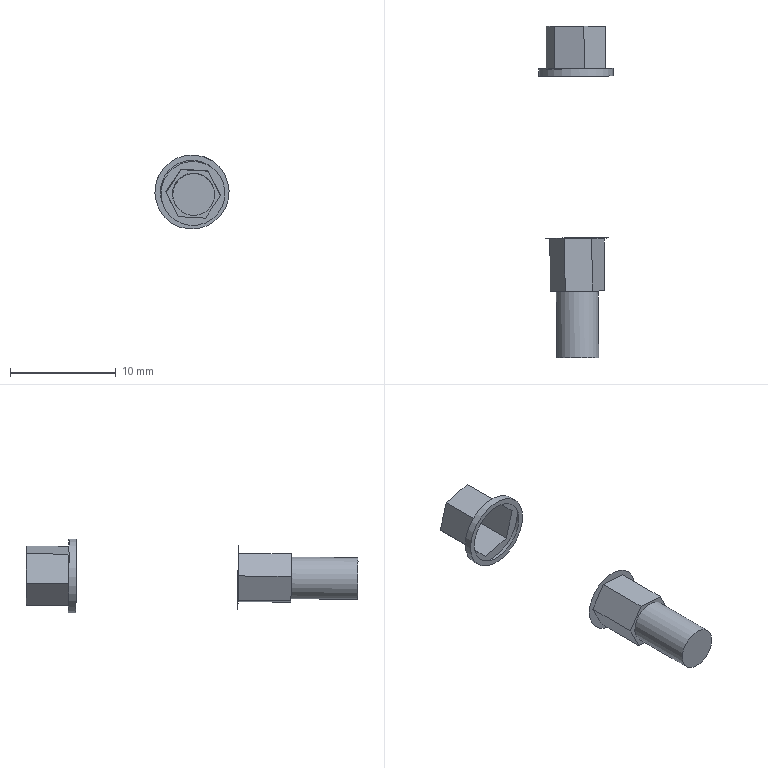Part | STEP file | Przeci_cie1[1] | 1 solid | 21 faces | box 7.004 x 31.35 x 7.006 mm | volume 710.625 mm3 | plane 18 | cylinder 2 | cone 1 | commonest cylinder face diameters 3.95 x1 7 x1
STEP:
#1=CARTESIAN_POINT('',(0.,0.,0.));
#2=DIRECTION('',(0.,0.,1.));
#3=DIRECTION('',(1.,0.,0.));
#4=AXIS2_PLACEMENT_3D('',#1,#2,#3);
#5=CARTESIAN_POINT('',(-96.81,-26.853,-116.249));
#6=VERTEX_POINT('',#5);
#7=CARTESIAN_POINT('',(-96.925,-11.554,-116.127));
#8=VERTEX_POINT('',#7);
#9=CARTESIAN_POINT('',(-96.81,-26.853,-116.249));
#10=DIRECTION('',(-0.007532,0.9999,0.007984));
#11=VECTOR('',#10,1.);
#12=LINE('',#9,#11);
#13=CARTESIAN_POINT('',(-99.446,-26.856,-117.722));
#14=DIRECTION('',(0.006008,-0.9999,-0.008835));
#15=DIRECTION('',(0.873,0.0009353,0.4878));
#16=AXIS2_PLACEMENT_3D('',#13,#14,#15);
#17=CONICAL_SURFACE('',#16,3.02,0.001745);
#18=CARTESIAN_POINT('',(0.,-0.000000001));
#19=DIRECTION('',(0.,-1.));
#20=VECTOR('',#19,1.);
#21=LINE('',#18,#20);
#22=(GEOMETRIC_REPRESENTATION_CONTEXT(2)PARAMETRIC_REPRESENTATION_CONTEXT()REPRESENTATION_CONTEXT('',''));
#23=DEFINITIONAL_REPRESENTATION('',(#21),#22);
#24=PCURVE('',#17,#23);
#25=CARTESIAN_POINT('',(6.283,-0.000000001));
#26=DIRECTION('',(0.,-1.));
#27=VECTOR('',#26,1.);
#28=LINE('',#25,#27);
#29=(GEOMETRIC_REPRESENTATION_CONTEXT(2)PARAMETRIC_REPRESENTATION_CONTEXT()REPRESENTATION_CONTEXT('',''));
#30=DEFINITIONAL_REPRESENTATION('',(#28),#29);
#31=PCURVE('',#17,#30);
#32=SEAM_CURVE('',#12,(#24,#31),.PCURVE_S1.);
#33=EDGE_CURVE('',#6,#8,#32,.T.);
#34=ORIENTED_EDGE('',*,*,#33,.T.);
#35=CARTESIAN_POINT('',(-99.538,-11.557,-117.587));
#36=DIRECTION('',(0.006008,-0.9999,-0.008835));
#37=DIRECTION('',(0.873,0.0009353,0.4878));
#38=AXIS2_PLACEMENT_3D('',#35,#36,#37);
#39=CIRCLE('',#38,2.993);
#40=CARTESIAN_POINT('',(0.000000001,-15.3));
#41=DIRECTION('',(1.,0.));
#42=VECTOR('',#41,1.);
#43=LINE('',#40,#42);
#44=(GEOMETRIC_REPRESENTATION_CONTEXT(2)PARAMETRIC_REPRESENTATION_CONTEXT()REPRESENTATION_CONTEXT('',''));
#45=DEFINITIONAL_REPRESENTATION('',(#43),#44);
#46=PCURVE('',#17,#45);
#47=CARTESIAN_POINT('',(-99.538,-11.557,-117.587));
#48=DIRECTION('',(-0.006008,0.9999,0.008835));
#49=DIRECTION('',(-0.873,-0.0009353,-0.4878));
#50=AXIS2_PLACEMENT_3D('',#47,#48,#49);
#51=PLANE('',#50);
#52=CARTESIAN_POINT('',(-2.993,0.));
#53=CARTESIAN_POINT('',(-2.993,5.185));
#54=CARTESIAN_POINT('',(1.497,2.592));
#55=CARTESIAN_POINT('',(5.987,0.));
#56=CARTESIAN_POINT('',(1.497,-2.592));
#57=CARTESIAN_POINT('',(-2.993,-5.185));
#58=CARTESIAN_POINT('',(-2.993,0.));
#59=(BOUNDED_CURVE()B_SPLINE_CURVE(2,(#52,#53,#54,#55,#56,#57,#58),.UNSPECIFIED.,.T.,.F.)B_SPLINE_CURVE_WITH_KNOTS((1,2,2,2,2,1),(-2.094,0.,2.094,4.189,6.283,8.378),.UNSPECIFIED.)CURVE()GEOMETRIC_REPRESENTATION_ITEM()RATIONAL_B_SPLINE_CURVE((1.,0.5,1.,0.5,1.,0.5,1.))REPRESENTATION_ITEM(''));
#60=(GEOMETRIC_REPRESENTATION_CONTEXT(2)PARAMETRIC_REPRESENTATION_CONTEXT()REPRESENTATION_CONTEXT('',''));
#61=DEFINITIONAL_REPRESENTATION('',(#59),#60);
#62=PCURVE('',#51,#61);
#63=SURFACE_CURVE('',#39,(#46,#62),.PCURVE_S1.);
#64=EDGE_CURVE('',#8,#8,#63,.T.);
#65=ORIENTED_EDGE('',*,*,#64,.T.);
#66=ORIENTED_EDGE('',*,*,#33,.F.);
#67=CARTESIAN_POINT('',(-99.446,-26.856,-117.722));
#68=DIRECTION('',(-0.006008,0.9999,0.008835));
#69=DIRECTION('',(0.873,0.0009353,0.4878));
#70=AXIS2_PLACEMENT_3D('',#67,#68,#69);
#71=CIRCLE('',#70,3.02);
#72=CARTESIAN_POINT('',(6.283,0.));
#73=DIRECTION('',(-1.,0.));
#74=VECTOR('',#73,1.);
#75=LINE('',#72,#74);
#76=(GEOMETRIC_REPRESENTATION_CONTEXT(2)PARAMETRIC_REPRESENTATION_CONTEXT()REPRESENTATION_CONTEXT('',''));
#77=DEFINITIONAL_REPRESENTATION('',(#75),#76);
#78=PCURVE('',#17,#77);
#79=CARTESIAN_POINT('',(-99.446,-26.856,-117.722));
#80=DIRECTION('',(0.006008,-0.9999,-0.008835));
#81=DIRECTION('',(0.873,0.0009353,0.4878));
#82=AXIS2_PLACEMENT_3D('',#79,#80,#81);
#83=PLANE('',#82);
#84=CARTESIAN_POINT('',(3.02,0.));
#85=CARTESIAN_POINT('',(3.02,-5.231));
#86=CARTESIAN_POINT('',(-1.51,-2.615));
#87=CARTESIAN_POINT('',(-6.04,0.));
#88=CARTESIAN_POINT('',(-1.51,2.615));
#89=CARTESIAN_POINT('',(3.02,5.231));
#90=CARTESIAN_POINT('',(3.02,0.));
#91=(BOUNDED_CURVE()B_SPLINE_CURVE(2,(#84,#85,#86,#87,#88,#89,#90),.UNSPECIFIED.,.T.,.F.)B_SPLINE_CURVE_WITH_KNOTS((1,2,2,2,2,1),(-2.094,0.,2.094,4.189,6.283,8.378),.UNSPECIFIED.)CURVE()GEOMETRIC_REPRESENTATION_ITEM()RATIONAL_B_SPLINE_CURVE((1.,0.5,1.,0.5,1.,0.5,1.))REPRESENTATION_ITEM(''));
#92=(GEOMETRIC_REPRESENTATION_CONTEXT(2)PARAMETRIC_REPRESENTATION_CONTEXT()REPRESENTATION_CONTEXT('',''));
#93=DEFINITIONAL_REPRESENTATION('',(#91),#92);
#94=PCURVE('',#83,#93);
#95=SURFACE_CURVE('',#71,(#78,#94),.PCURVE_S1.);
#96=EDGE_CURVE('',#6,#6,#95,.T.);
#97=ORIENTED_EDGE('',*,*,#96,.T.);
#98=EDGE_LOOP('',(#34,#65,#66,#97));
#99=FACE_BOUND('',#98,.T.);
#100=ADVANCED_FACE('',(#99),#17,.T.);
#101=CARTESIAN_POINT('',(-102.598,-10.86,-119.288));
#102=VERTEX_POINT('',#101);
#103=CARTESIAN_POINT('',(-102.594,-11.56,-119.294));
#104=VERTEX_POINT('',#103);
#105=CARTESIAN_POINT('',(-102.598,-10.86,-119.288));
#106=DIRECTION('',(0.006008,-0.9999,-0.008835));
#107=VECTOR('',#106,1.);
#108=LINE('',#105,#107);
#109=CARTESIAN_POINT('',(-99.538,-11.557,-117.587));
#110=DIRECTION('',(-0.006008,0.9999,0.008835));
#111=DIRECTION('',(-0.873,-0.0009353,-0.4878));
#112=AXIS2_PLACEMENT_3D('',#109,#110,#111);
#113=CYLINDRICAL_SURFACE('',#112,3.5);
#114=CARTESIAN_POINT('',(0.,0.7));
#115=DIRECTION('',(0.,-1.));
#116=VECTOR('',#115,1.);
#117=LINE('',#114,#116);
#118=(GEOMETRIC_REPRESENTATION_CONTEXT(2)PARAMETRIC_REPRESENTATION_CONTEXT()REPRESENTATION_CONTEXT('',''));
#119=DEFINITIONAL_REPRESENTATION('',(#117),#118);
#120=PCURVE('',#113,#119);
#121=CARTESIAN_POINT('',(6.283,0.7));
#122=DIRECTION('',(0.,-1.));
#123=VECTOR('',#122,1.);
#124=LINE('',#121,#123);
#125=(GEOMETRIC_REPRESENTATION_CONTEXT(2)PARAMETRIC_REPRESENTATION_CONTEXT()REPRESENTATION_CONTEXT('',''));
#126=DEFINITIONAL_REPRESENTATION('',(#124),#125);
#127=PCURVE('',#113,#126);
#128=SEAM_CURVE('',#108,(#120,#127),.PCURVE_S1.);
#129=EDGE_CURVE('',#102,#104,#128,.T.);
#130=ORIENTED_EDGE('',*,*,#129,.T.);
#131=CARTESIAN_POINT('',(-99.538,-11.557,-117.587));
#132=DIRECTION('',(-0.006008,0.9999,0.008835));
#133=DIRECTION('',(-0.873,-0.0009353,-0.4878));
#134=AXIS2_PLACEMENT_3D('',#131,#132,#133);
#135=CIRCLE('',#134,3.5);
#136=CARTESIAN_POINT('',(0.,0.));
#137=DIRECTION('',(1.,0.));
#138=VECTOR('',#137,1.);
#139=LINE('',#136,#138);
#140=(GEOMETRIC_REPRESENTATION_CONTEXT(2)PARAMETRIC_REPRESENTATION_CONTEXT()REPRESENTATION_CONTEXT('',''));
#141=DEFINITIONAL_REPRESENTATION('',(#139),#140);
#142=PCURVE('',#113,#141);
#143=CARTESIAN_POINT('',(0.,0.));
#144=DIRECTION('',(1.,0.));
#145=AXIS2_PLACEMENT_2D('',#143,#144);
#146=CIRCLE('',#145,3.5);
#147=(GEOMETRIC_REPRESENTATION_CONTEXT(2)PARAMETRIC_REPRESENTATION_CONTEXT()REPRESENTATION_CONTEXT('',''));
#148=DEFINITIONAL_REPRESENTATION('',(#146),#147);
#149=PCURVE('',#51,#148);
#150=SURFACE_CURVE('',#135,(#142,#149),.PCURVE_S1.);
#151=EDGE_CURVE('',#104,#104,#150,.T.);
#152=ORIENTED_EDGE('',*,*,#151,.T.);
#153=ORIENTED_EDGE('',*,*,#129,.F.);
#154=CARTESIAN_POINT('',(-99.542,-10.857,-117.581));
#155=DIRECTION('',(0.006008,-0.9999,-0.008835));
#156=DIRECTION('',(-0.873,-0.0009353,-0.4878));
#157=AXIS2_PLACEMENT_3D('',#154,#155,#156);
#158=CIRCLE('',#157,3.5);
#159=CARTESIAN_POINT('',(6.283,0.7));
#160=DIRECTION('',(-1.,0.));
#161=VECTOR('',#160,1.);
#162=LINE('',#159,#161);
#163=(GEOMETRIC_REPRESENTATION_CONTEXT(2)PARAMETRIC_REPRESENTATION_CONTEXT()REPRESENTATION_CONTEXT('',''));
#164=DEFINITIONAL_REPRESENTATION('',(#162),#163);
#165=PCURVE('',#113,#164);
#166=CARTESIAN_POINT('',(-99.542,-10.857,-117.581));
#167=DIRECTION('',(-0.006008,0.9999,0.008835));
#168=DIRECTION('',(-0.873,-0.0009353,-0.4878));
#169=AXIS2_PLACEMENT_3D('',#166,#167,#168);
#170=PLANE('',#169);
#171=CARTESIAN_POINT('',(3.5,0.));
#172=CARTESIAN_POINT('',(3.5,-6.062));
#173=CARTESIAN_POINT('',(-1.75,-3.031));
#174=CARTESIAN_POINT('',(-7.,0.));
#175=CARTESIAN_POINT('',(-1.75,3.031));
#176=CARTESIAN_POINT('',(3.5,6.062));
#177=CARTESIAN_POINT('',(3.5,0.));
#178=(BOUNDED_CURVE()B_SPLINE_CURVE(2,(#171,#172,#173,#174,#175,#176,#177),.UNSPECIFIED.,.T.,.F.)B_SPLINE_CURVE_WITH_KNOTS((1,2,2,2,2,1),(-2.094,0.,2.094,4.189,6.283,8.378),.UNSPECIFIED.)CURVE()GEOMETRIC_REPRESENTATION_ITEM()RATIONAL_B_SPLINE_CURVE((1.,0.5,1.,0.5,1.,0.5,1.))REPRESENTATION_ITEM(''));
#179=(GEOMETRIC_REPRESENTATION_CONTEXT(2)PARAMETRIC_REPRESENTATION_CONTEXT()REPRESENTATION_CONTEXT('',''));
#180=DEFINITIONAL_REPRESENTATION('',(#178),#179);
#181=PCURVE('',#170,#180);
#182=SURFACE_CURVE('',#158,(#165,#181),.PCURVE_S1.);
#183=EDGE_CURVE('',#102,#102,#182,.T.);
#184=ORIENTED_EDGE('',*,*,#183,.T.);
#185=EDGE_LOOP('',(#130,#152,#153,#184));
#186=FACE_BOUND('',#185,.T.);
#187=ADVANCED_FACE('',(#186),#113,.T.);
#188=CARTESIAN_POINT('',(-101.14,-31.857,-118.729));
#189=VERTEX_POINT('',#188);
#190=CARTESIAN_POINT('',(-101.102,-38.157,-118.785));
#191=VERTEX_POINT('',#190);
#192=CARTESIAN_POINT('',(-101.14,-31.857,-118.729));
#193=DIRECTION('',(0.006008,-0.9999,-0.008835));
#194=VECTOR('',#193,1.);
#195=LINE('',#192,#194);
#196=CARTESIAN_POINT('',(-99.378,-38.155,-117.822));
#197=DIRECTION('',(-0.006008,0.9999,0.008835));
#198=DIRECTION('',(-0.873,-0.0009353,-0.4878));
#199=AXIS2_PLACEMENT_3D('',#196,#197,#198);
#200=CYLINDRICAL_SURFACE('',#199,1.975);
#201=CARTESIAN_POINT('',(0.,6.3));
#202=DIRECTION('',(0.,-1.));
#203=VECTOR('',#202,1.);
#204=LINE('',#201,#203);
#205=(GEOMETRIC_REPRESENTATION_CONTEXT(2)PARAMETRIC_REPRESENTATION_CONTEXT()REPRESENTATION_CONTEXT('',''));
#206=DEFINITIONAL_REPRESENTATION('',(#204),#205);
#207=PCURVE('',#200,#206);
#208=CARTESIAN_POINT('',(6.283,6.3));
#209=DIRECTION('',(0.,-1.));
#210=VECTOR('',#209,1.);
#211=LINE('',#208,#210);
#212=(GEOMETRIC_REPRESENTATION_CONTEXT(2)PARAMETRIC_REPRESENTATION_CONTEXT()REPRESENTATION_CONTEXT('',''));
#213=DEFINITIONAL_REPRESENTATION('',(#211),#212);
#214=PCURVE('',#200,#213);
#215=SEAM_CURVE('',#195,(#207,#214),.PCURVE_S1.);
#216=EDGE_CURVE('',#189,#191,#215,.T.);
#217=ORIENTED_EDGE('',*,*,#216,.T.);
#218=CARTESIAN_POINT('',(-99.378,-38.155,-117.822));
#219=DIRECTION('',(-0.006008,0.9999,0.008835));
#220=DIRECTION('',(-0.873,-0.0009353,-0.4878));
#221=AXIS2_PLACEMENT_3D('',#218,#219,#220);
#222=CIRCLE('',#221,1.975);
#223=CARTESIAN_POINT('',(0.,0.));
#224=DIRECTION('',(1.,0.));
#225=VECTOR('',#224,1.);
#226=LINE('',#223,#225);
#227=(GEOMETRIC_REPRESENTATION_CONTEXT(2)PARAMETRIC_REPRESENTATION_CONTEXT()REPRESENTATION_CONTEXT('',''));
#228=DEFINITIONAL_REPRESENTATION('',(#226),#227);
#229=PCURVE('',#200,#228);
#230=CARTESIAN_POINT('',(-99.378,-38.155,-117.822));
#231=DIRECTION('',(0.006008,-0.9999,-0.008835));
#232=DIRECTION('',(0.873,0.0009353,0.4878));
#233=AXIS2_PLACEMENT_3D('',#230,#231,#232);
#234=PLANE('',#233);
#235=CARTESIAN_POINT('',(-1.975,0.));
#236=CARTESIAN_POINT('',(-1.975,3.421));
#237=CARTESIAN_POINT('',(0.9875,1.71));
#238=CARTESIAN_POINT('',(3.95,0.));
#239=CARTESIAN_POINT('',(0.9875,-1.71));
#240=CARTESIAN_POINT('',(-1.975,-3.421));
#241=CARTESIAN_POINT('',(-1.975,0.));
#242=(BOUNDED_CURVE()B_SPLINE_CURVE(2,(#235,#236,#237,#238,#239,#240,#241),.UNSPECIFIED.,.T.,.F.)B_SPLINE_CURVE_WITH_KNOTS((1,2,2,2,2,1),(-2.094,0.,2.094,4.189,6.283,8.378),.UNSPECIFIED.)CURVE()GEOMETRIC_REPRESENTATION_ITEM()RATIONAL_B_SPLINE_CURVE((1.,0.5,1.,0.5,1.,0.5,1.))REPRESENTATION_ITEM(''));
#243=(GEOMETRIC_REPRESENTATION_CONTEXT(2)PARAMETRIC_REPRESENTATION_CONTEXT()REPRESENTATION_CONTEXT('',''));
#244=DEFINITIONAL_REPRESENTATION('',(#242),#243);
#245=PCURVE('',#234,#244);
#246=SURFACE_CURVE('',#222,(#229,#245),.PCURVE_S1.);
#247=EDGE_CURVE('',#191,#191,#246,.T.);
#248=ORIENTED_EDGE('',*,*,#247,.T.);
#249=ORIENTED_EDGE('',*,*,#216,.F.);
#250=CARTESIAN_POINT('',(-99.416,-31.856,-117.766));
#251=DIRECTION('',(-0.006008,0.9999,0.008835));
#252=DIRECTION('',(-0.873,-0.0009353,-0.4878));
#253=AXIS2_PLACEMENT_3D('',#250,#251,#252);
#254=CIRCLE('',#253,1.975);
#255=CARTESIAN_POINT('',(0.,6.3));
#256=DIRECTION('',(1.,0.));
#257=VECTOR('',#256,1.);
#258=LINE('',#255,#257);
#259=(GEOMETRIC_REPRESENTATION_CONTEXT(2)PARAMETRIC_REPRESENTATION_CONTEXT()REPRESENTATION_CONTEXT('',''));
#260=DEFINITIONAL_REPRESENTATION('',(#258),#259);
#261=PCURVE('',#200,#260);
#262=CARTESIAN_POINT('',(-99.416,-31.856,-117.766));
#263=DIRECTION('',(0.006008,-0.9999,-0.008835));
#264=DIRECTION('',(0.873,0.0009353,0.4878));
#265=AXIS2_PLACEMENT_3D('',#262,#263,#264);
#266=PLANE('',#265);
#267=CARTESIAN_POINT('',(-1.975,0.));
#268=CARTESIAN_POINT('',(-1.975,3.421));
#269=CARTESIAN_POINT('',(0.9875,1.71));
#270=CARTESIAN_POINT('',(3.95,0.));
#271=CARTESIAN_POINT('',(0.9875,-1.71));
#272=CARTESIAN_POINT('',(-1.975,-3.421));
#273=CARTESIAN_POINT('',(-1.975,0.));
#274=(BOUNDED_CURVE()B_SPLINE_CURVE(2,(#267,#268,#269,#270,#271,#272,#273),.UNSPECIFIED.,.T.,.F.)B_SPLINE_CURVE_WITH_KNOTS((1,2,2,2,2,1),(-2.094,0.,2.094,4.189,6.283,8.378),.UNSPECIFIED.)CURVE()GEOMETRIC_REPRESENTATION_ITEM()RATIONAL_B_SPLINE_CURVE((1.,0.5,1.,0.5,1.,0.5,1.))REPRESENTATION_ITEM(''));
#275=(GEOMETRIC_REPRESENTATION_CONTEXT(2)PARAMETRIC_REPRESENTATION_CONTEXT()REPRESENTATION_CONTEXT('',''));
#276=DEFINITIONAL_REPRESENTATION('',(#274),#275);
#277=PCURVE('',#266,#276);
#278=SURFACE_CURVE('',#254,(#261,#277),.PCURVE_S1.);
#279=EDGE_CURVE('',#189,#189,#278,.T.);
#280=ORIENTED_EDGE('',*,*,#279,.F.);
#281=EDGE_LOOP('',(#217,#248,#249,#280));
#282=FACE_BOUND('',#281,.T.);
#283=ADVANCED_FACE('',(#282),#200,.T.);
#284=ORIENTED_EDGE('',*,*,#64,.F.);
#285=EDGE_LOOP('',(#284));
#286=FACE_BOUND('',#285,.T.);
#287=ORIENTED_EDGE('',*,*,#151,.F.);
#288=EDGE_LOOP('',(#287));
#289=FACE_BOUND('',#288,.T.);
#290=ADVANCED_FACE('',(#286,#289),#51,.F.);
#291=CARTESIAN_POINT('',(-102.006,-26.873,-117.578));
#292=VERTEX_POINT('',#291);
#293=CARTESIAN_POINT('',(-100.601,-26.883,-115.433));
#294=VERTEX_POINT('',#293);
#295=CARTESIAN_POINT('',(-102.006,-26.873,-117.578));
#296=DIRECTION('',(0.5479,-0.004099,0.8365));
#297=VECTOR('',#296,1.);
#298=LINE('',#295,#297);
#299=CARTESIAN_POINT('',(-2.164,1.374));
#300=DIRECTION('',(0.8864,0.463));
#301=VECTOR('',#300,1.);
#302=LINE('',#299,#301);
#303=(GEOMETRIC_REPRESENTATION_CONTEXT(2)PARAMETRIC_REPRESENTATION_CONTEXT()REPRESENTATION_CONTEXT('',''));
#304=DEFINITIONAL_REPRESENTATION('',(#302),#303);
#305=PCURVE('',#83,#304);
#306=CARTESIAN_POINT('',(-101.288,-29.378,-116.528));
#307=DIRECTION('',(0.8365,0.009867,-0.5479));
#308=DIRECTION('',(0.5479,-0.004099,0.8365));
#309=AXIS2_PLACEMENT_3D('',#306,#307,#308);
#310=PLANE('',#309);
#311=CARTESIAN_POINT('',(-1.282,-2.5));
#312=DIRECTION('',(1.,0.));
#313=VECTOR('',#312,1.);
#314=LINE('',#311,#313);
#315=(GEOMETRIC_REPRESENTATION_CONTEXT(2)PARAMETRIC_REPRESENTATION_CONTEXT()REPRESENTATION_CONTEXT('',''));
#316=DEFINITIONAL_REPRESENTATION('',(#314),#315);
#317=PCURVE('',#310,#316);
#318=SURFACE_CURVE('',#298,(#305,#317),.PCURVE_S1.);
#319=EDGE_CURVE('',#292,#294,#318,.T.);
#320=ORIENTED_EDGE('',*,*,#319,.T.);
#321=CARTESIAN_POINT('',(-98.042,-26.866,-115.578));
#322=VERTEX_POINT('',#321);
#323=CARTESIAN_POINT('',(-100.601,-26.883,-115.433));
#324=DIRECTION('',(0.9984,0.006496,-0.05624));
#325=VECTOR('',#324,1.);
#326=LINE('',#323,#325);
#327=CARTESIAN_POINT('',(0.1083,2.561));
#328=DIRECTION('',(0.8441,-0.5361));
#329=VECTOR('',#328,1.);
#330=LINE('',#327,#329);
#331=(GEOMETRIC_REPRESENTATION_CONTEXT(2)PARAMETRIC_REPRESENTATION_CONTEXT()REPRESENTATION_CONTEXT('',''));
#332=DEFINITIONAL_REPRESENTATION('',(#330),#331);
#333=PCURVE('',#83,#332);
#334=CARTESIAN_POINT('',(-99.306,-29.375,-115.528));
#335=DIRECTION('',(-0.05629,0.008483,-0.9984));
#336=DIRECTION('',(0.9984,0.006496,-0.05624));
#337=AXIS2_PLACEMENT_3D('',#334,#335,#336);
#338=PLANE('',#337);
#339=CARTESIAN_POINT('',(-1.282,-2.5));
#340=DIRECTION('',(1.,0.));
#341=VECTOR('',#340,1.);
#342=LINE('',#339,#341);
#343=(GEOMETRIC_REPRESENTATION_CONTEXT(2)PARAMETRIC_REPRESENTATION_CONTEXT()REPRESENTATION_CONTEXT('',''));
#344=DEFINITIONAL_REPRESENTATION('',(#342),#343);
#345=PCURVE('',#338,#344);
#346=SURFACE_CURVE('',#326,(#333,#345),.PCURVE_S1.);
#347=EDGE_CURVE('',#294,#322,#346,.T.);
#348=ORIENTED_EDGE('',*,*,#347,.T.);
#349=CARTESIAN_POINT('',(-96.887,-26.839,-117.866));
#350=VERTEX_POINT('',#349);
#351=CARTESIAN_POINT('',(-98.042,-26.866,-115.578));
#352=DIRECTION('',(0.4504,0.01059,-0.8927));
#353=VECTOR('',#352,1.);
#354=LINE('',#351,#353);
#355=CARTESIAN_POINT('',(2.272,1.187));
#356=DIRECTION('',(-0.04224,-0.9991));
#357=VECTOR('',#356,1.);
#358=LINE('',#355,#357);
#359=(GEOMETRIC_REPRESENTATION_CONTEXT(2)PARAMETRIC_REPRESENTATION_CONTEXT()REPRESENTATION_CONTEXT('',''));
#360=DEFINITIONAL_REPRESENTATION('',(#358),#359);
#361=PCURVE('',#83,#360);
#362=CARTESIAN_POINT('',(-97.449,-29.353,-116.744));
#363=DIRECTION('',(-0.8928,-0.001384,-0.4505));
#364=DIRECTION('',(0.4504,0.01059,-0.8927));
#365=AXIS2_PLACEMENT_3D('',#362,#363,#364);
#366=PLANE('',#365);
#367=CARTESIAN_POINT('',(-1.282,-2.5));
#368=DIRECTION('',(1.,0.));
#369=VECTOR('',#368,1.);
#370=LINE('',#367,#369);
#371=(GEOMETRIC_REPRESENTATION_CONTEXT(2)PARAMETRIC_REPRESENTATION_CONTEXT()REPRESENTATION_CONTEXT('',''));
#372=DEFINITIONAL_REPRESENTATION('',(#370),#371);
#373=PCURVE('',#366,#372);
#374=SURFACE_CURVE('',#354,(#361,#373),.PCURVE_S1.);
#375=EDGE_CURVE('',#322,#350,#374,.T.);
#376=ORIENTED_EDGE('',*,*,#375,.T.);
#377=CARTESIAN_POINT('',(-98.292,-26.829,-120.01));
#378=VERTEX_POINT('',#377);
#379=CARTESIAN_POINT('',(-96.887,-26.839,-117.866));
#380=DIRECTION('',(-0.5479,0.004099,-0.8365));
#381=VECTOR('',#380,1.);
#382=LINE('',#379,#381);
#383=CARTESIAN_POINT('',(2.164,-1.374));
#384=DIRECTION('',(-0.8864,-0.463));
#385=VECTOR('',#384,1.);
#386=LINE('',#383,#385);
#387=(GEOMETRIC_REPRESENTATION_CONTEXT(2)PARAMETRIC_REPRESENTATION_CONTEXT()REPRESENTATION_CONTEXT('',''));
#388=DEFINITIONAL_REPRESENTATION('',(#386),#387);
#389=PCURVE('',#83,#388);
#390=CARTESIAN_POINT('',(-97.574,-29.334,-118.96));
#391=DIRECTION('',(-0.8365,-0.009867,0.5479));
#392=DIRECTION('',(-0.5479,0.004099,-0.8365));
#393=AXIS2_PLACEMENT_3D('',#390,#391,#392);
#394=PLANE('',#393);
#395=CARTESIAN_POINT('',(-1.282,-2.5));
#396=DIRECTION('',(1.,0.));
#397=VECTOR('',#396,1.);
#398=LINE('',#395,#397);
#399=(GEOMETRIC_REPRESENTATION_CONTEXT(2)PARAMETRIC_REPRESENTATION_CONTEXT()REPRESENTATION_CONTEXT('',''));
#400=DEFINITIONAL_REPRESENTATION('',(#398),#399);
#401=PCURVE('',#394,#400);
#402=SURFACE_CURVE('',#382,(#389,#401),.PCURVE_S1.);
#403=EDGE_CURVE('',#350,#378,#402,.T.);
#404=ORIENTED_EDGE('',*,*,#403,.T.);
#405=CARTESIAN_POINT('',(-100.851,-26.845,-119.866));
#406=VERTEX_POINT('',#405);
#407=CARTESIAN_POINT('',(-98.292,-26.829,-120.01));
#408=DIRECTION('',(-0.9984,-0.006496,0.05624));
#409=VECTOR('',#408,1.);
#410=LINE('',#407,#409);
#411=CARTESIAN_POINT('',(-0.1083,-2.561));
#412=DIRECTION('',(-0.8441,0.5361));
#413=VECTOR('',#412,1.);
#414=LINE('',#411,#413);
#415=(GEOMETRIC_REPRESENTATION_CONTEXT(2)PARAMETRIC_REPRESENTATION_CONTEXT()REPRESENTATION_CONTEXT('',''));
#416=DEFINITIONAL_REPRESENTATION('',(#414),#415);
#417=PCURVE('',#83,#416);
#418=CARTESIAN_POINT('',(-99.556,-29.337,-119.96));
#419=DIRECTION('',(0.05629,-0.008483,0.9984));
#420=DIRECTION('',(-0.9984,-0.006496,0.05624));
#421=AXIS2_PLACEMENT_3D('',#418,#419,#420);
#422=PLANE('',#421);
#423=CARTESIAN_POINT('',(-1.282,-2.5));
#424=DIRECTION('',(1.,0.));
#425=VECTOR('',#424,1.);
#426=LINE('',#423,#425);
#427=(GEOMETRIC_REPRESENTATION_CONTEXT(2)PARAMETRIC_REPRESENTATION_CONTEXT()REPRESENTATION_CONTEXT('',''));
#428=DEFINITIONAL_REPRESENTATION('',(#426),#427);
#429=PCURVE('',#422,#428);
#430=SURFACE_CURVE('',#410,(#417,#429),.PCURVE_S1.);
#431=EDGE_CURVE('',#378,#406,#430,.T.);
#432=ORIENTED_EDGE('',*,*,#431,.T.);
#433=CARTESIAN_POINT('',(-100.851,-26.845,-119.866));
#434=DIRECTION('',(-0.4504,-0.01059,0.8927));
#435=VECTOR('',#434,1.);
#436=LINE('',#433,#435);
#437=CARTESIAN_POINT('',(-2.272,-1.187));
#438=DIRECTION('',(0.04224,0.9991));
#439=VECTOR('',#438,1.);
#440=LINE('',#437,#439);
#441=(GEOMETRIC_REPRESENTATION_CONTEXT(2)PARAMETRIC_REPRESENTATION_CONTEXT()REPRESENTATION_CONTEXT('',''));
#442=DEFINITIONAL_REPRESENTATION('',(#440),#441);
#443=PCURVE('',#83,#442);
#444=CARTESIAN_POINT('',(-101.413,-29.359,-118.744));
#445=DIRECTION('',(0.8928,0.001384,0.4505));
#446=DIRECTION('',(-0.4504,-0.01059,0.8927));
#447=AXIS2_PLACEMENT_3D('',#444,#445,#446);
#448=PLANE('',#447);
#449=CARTESIAN_POINT('',(-1.282,-2.5));
#450=DIRECTION('',(1.,0.));
#451=VECTOR('',#450,1.);
#452=LINE('',#449,#451);
#453=(GEOMETRIC_REPRESENTATION_CONTEXT(2)PARAMETRIC_REPRESENTATION_CONTEXT()REPRESENTATION_CONTEXT('',''));
#454=DEFINITIONAL_REPRESENTATION('',(#452),#453);
#455=PCURVE('',#448,#454);
#456=SURFACE_CURVE('',#436,(#443,#455),.PCURVE_S1.);
#457=EDGE_CURVE('',#406,#292,#456,.T.);
#458=ORIENTED_EDGE('',*,*,#457,.T.);
#459=EDGE_LOOP('',(#320,#348,#376,#404,#432,#458));
#460=FACE_BOUND('',#459,.T.);
#461=ORIENTED_EDGE('',*,*,#96,.F.);
#462=EDGE_LOOP('',(#461));
#463=FACE_BOUND('',#462,.T.);
#464=ADVANCED_FACE('',(#460,#463),#83,.T.);
#465=CARTESIAN_POINT('',(-100.571,-31.883,-115.478));
#466=VERTEX_POINT('',#465);
#467=CARTESIAN_POINT('',(-100.571,-31.883,-115.478));
#468=DIRECTION('',(-0.006008,0.9999,0.008835));
#469=VECTOR('',#468,1.);
#470=LINE('',#467,#469);
#471=CARTESIAN_POINT('',(-1.282,2.5));
#472=DIRECTION('',(0.,-1.));
#473=VECTOR('',#472,1.);
#474=LINE('',#471,#473);
#475=(GEOMETRIC_REPRESENTATION_CONTEXT(2)PARAMETRIC_REPRESENTATION_CONTEXT()REPRESENTATION_CONTEXT('',''));
#476=DEFINITIONAL_REPRESENTATION('',(#474),#475);
#477=PCURVE('',#338,#476);
#478=CARTESIAN_POINT('',(1.282,2.5));
#479=DIRECTION('',(0.,-1.));
#480=VECTOR('',#479,1.);
#481=LINE('',#478,#480);
#482=(GEOMETRIC_REPRESENTATION_CONTEXT(2)PARAMETRIC_REPRESENTATION_CONTEXT()REPRESENTATION_CONTEXT('',''));
#483=DEFINITIONAL_REPRESENTATION('',(#481),#482);
#484=PCURVE('',#310,#483);
#485=SURFACE_CURVE('',#470,(#477,#484),.PCURVE_S1.);
#486=EDGE_CURVE('',#466,#294,#485,.T.);
#487=ORIENTED_EDGE('',*,*,#486,.F.);
#488=CARTESIAN_POINT('',(-98.012,-31.866,-115.622));
#489=VERTEX_POINT('',#488);
#490=CARTESIAN_POINT('',(-98.012,-31.866,-115.622));
#491=DIRECTION('',(-0.9984,-0.006496,0.05624));
#492=VECTOR('',#491,1.);
#493=LINE('',#490,#492);
#494=CARTESIAN_POINT('',(1.282,2.5));
#495=DIRECTION('',(-1.,0.));
#496=VECTOR('',#495,1.);
#497=LINE('',#494,#496);
#498=(GEOMETRIC_REPRESENTATION_CONTEXT(2)PARAMETRIC_REPRESENTATION_CONTEXT()REPRESENTATION_CONTEXT('',''));
#499=DEFINITIONAL_REPRESENTATION('',(#497),#498);
#500=PCURVE('',#338,#499);
#501=CARTESIAN_POINT('',(2.272,1.187));
#502=DIRECTION('',(-0.8441,0.5361));
#503=VECTOR('',#502,1.);
#504=LINE('',#501,#503);
#505=(GEOMETRIC_REPRESENTATION_CONTEXT(2)PARAMETRIC_REPRESENTATION_CONTEXT()REPRESENTATION_CONTEXT('',''));
#506=DEFINITIONAL_REPRESENTATION('',(#504),#505);
#507=PCURVE('',#266,#506);
#508=SURFACE_CURVE('',#493,(#500,#507),.PCURVE_S1.);
#509=EDGE_CURVE('',#489,#466,#508,.T.);
#510=ORIENTED_EDGE('',*,*,#509,.F.);
#511=CARTESIAN_POINT('',(-98.042,-26.866,-115.578));
#512=DIRECTION('',(0.006008,-0.9999,-0.008835));
#513=VECTOR('',#512,1.);
#514=LINE('',#511,#513);
#515=CARTESIAN_POINT('',(1.282,-2.5));
#516=DIRECTION('',(0.,1.));
#517=VECTOR('',#516,1.);
#518=LINE('',#515,#517);
#519=(GEOMETRIC_REPRESENTATION_CONTEXT(2)PARAMETRIC_REPRESENTATION_CONTEXT()REPRESENTATION_CONTEXT('',''));
#520=DEFINITIONAL_REPRESENTATION('',(#518),#519);
#521=PCURVE('',#338,#520);
#522=CARTESIAN_POINT('',(-1.282,-2.5));
#523=DIRECTION('',(0.,1.));
#524=VECTOR('',#523,1.);
#525=LINE('',#522,#524);
#526=(GEOMETRIC_REPRESENTATION_CONTEXT(2)PARAMETRIC_REPRESENTATION_CONTEXT()REPRESENTATION_CONTEXT('',''));
#527=DEFINITIONAL_REPRESENTATION('',(#525),#526);
#528=PCURVE('',#366,#527);
#529=SURFACE_CURVE('',#514,(#521,#528),.PCURVE_S1.);
#530=EDGE_CURVE('',#322,#489,#529,.T.);
#531=ORIENTED_EDGE('',*,*,#530,.F.);
#532=ORIENTED_EDGE('',*,*,#347,.F.);
#533=EDGE_LOOP('',(#487,#510,#531,#532));
#534=FACE_BOUND('',#533,.T.);
#535=ADVANCED_FACE('',(#534),#338,.F.);
#536=CARTESIAN_POINT('',(-101.976,-31.872,-117.622));
#537=VERTEX_POINT('',#536);
#538=CARTESIAN_POINT('',(-101.976,-31.872,-117.622));
#539=DIRECTION('',(-0.006008,0.9999,0.008835));
#540=VECTOR('',#539,1.);
#541=LINE('',#538,#540);
#542=CARTESIAN_POINT('',(-1.282,2.5));
#543=DIRECTION('',(0.,-1.));
#544=VECTOR('',#543,1.);
#545=LINE('',#542,#544);
#546=(GEOMETRIC_REPRESENTATION_CONTEXT(2)PARAMETRIC_REPRESENTATION_CONTEXT()REPRESENTATION_CONTEXT('',''));
#547=DEFINITIONAL_REPRESENTATION('',(#545),#546);
#548=PCURVE('',#310,#547);
#549=CARTESIAN_POINT('',(1.282,2.5));
#550=DIRECTION('',(0.,-1.));
#551=VECTOR('',#550,1.);
#552=LINE('',#549,#551);
#553=(GEOMETRIC_REPRESENTATION_CONTEXT(2)PARAMETRIC_REPRESENTATION_CONTEXT()REPRESENTATION_CONTEXT('',''));
#554=DEFINITIONAL_REPRESENTATION('',(#552),#553);
#555=PCURVE('',#448,#554);
#556=SURFACE_CURVE('',#541,(#548,#555),.PCURVE_S1.);
#557=EDGE_CURVE('',#537,#292,#556,.T.);
#558=ORIENTED_EDGE('',*,*,#557,.F.);
#559=CARTESIAN_POINT('',(-100.571,-31.883,-115.478));
#560=DIRECTION('',(-0.5479,0.004099,-0.8365));
#561=VECTOR('',#560,1.);
#562=LINE('',#559,#561);
#563=CARTESIAN_POINT('',(1.282,2.5));
#564=DIRECTION('',(-1.,0.));
#565=VECTOR('',#564,1.);
#566=LINE('',#563,#565);
#567=(GEOMETRIC_REPRESENTATION_CONTEXT(2)PARAMETRIC_REPRESENTATION_CONTEXT()REPRESENTATION_CONTEXT('',''));
#568=DEFINITIONAL_REPRESENTATION('',(#566),#567);
#569=PCURVE('',#310,#568);
#570=CARTESIAN_POINT('',(0.1083,2.561));
#571=DIRECTION('',(-0.8864,-0.463));
#572=VECTOR('',#571,1.);
#573=LINE('',#570,#572);
#574=(GEOMETRIC_REPRESENTATION_CONTEXT(2)PARAMETRIC_REPRESENTATION_CONTEXT()REPRESENTATION_CONTEXT('',''));
#575=DEFINITIONAL_REPRESENTATION('',(#573),#574);
#576=PCURVE('',#266,#575);
#577=SURFACE_CURVE('',#562,(#569,#576),.PCURVE_S1.);
#578=EDGE_CURVE('',#466,#537,#577,.T.);
#579=ORIENTED_EDGE('',*,*,#578,.F.);
#580=ORIENTED_EDGE('',*,*,#486,.T.);
#581=ORIENTED_EDGE('',*,*,#319,.F.);
#582=EDGE_LOOP('',(#558,#579,#580,#581));
#583=FACE_BOUND('',#582,.T.);
#584=ADVANCED_FACE('',(#583),#310,.F.);
#585=CARTESIAN_POINT('',(-100.821,-31.845,-119.91));
#586=VERTEX_POINT('',#585);
#587=CARTESIAN_POINT('',(-100.821,-31.845,-119.91));
#588=DIRECTION('',(-0.006008,0.9999,0.008835));
#589=VECTOR('',#588,1.);
#590=LINE('',#587,#589);
#591=CARTESIAN_POINT('',(-1.282,2.5));
#592=DIRECTION('',(0.,-1.));
#593=VECTOR('',#592,1.);
#594=LINE('',#591,#593);
#595=(GEOMETRIC_REPRESENTATION_CONTEXT(2)PARAMETRIC_REPRESENTATION_CONTEXT()REPRESENTATION_CONTEXT('',''));
#596=DEFINITIONAL_REPRESENTATION('',(#594),#595);
#597=PCURVE('',#448,#596);
#598=CARTESIAN_POINT('',(1.282,2.5));
#599=DIRECTION('',(0.,-1.));
#600=VECTOR('',#599,1.);
#601=LINE('',#598,#600);
#602=(GEOMETRIC_REPRESENTATION_CONTEXT(2)PARAMETRIC_REPRESENTATION_CONTEXT()REPRESENTATION_CONTEXT('',''));
#603=DEFINITIONAL_REPRESENTATION('',(#601),#602);
#604=PCURVE('',#422,#603);
#605=SURFACE_CURVE('',#590,(#597,#604),.PCURVE_S1.);
#606=EDGE_CURVE('',#586,#406,#605,.T.);
#607=ORIENTED_EDGE('',*,*,#606,.F.);
#608=CARTESIAN_POINT('',(-101.976,-31.872,-117.622));
#609=DIRECTION('',(0.4504,0.01059,-0.8927));
#610=VECTOR('',#609,1.);
#611=LINE('',#608,#610);
#612=CARTESIAN_POINT('',(1.282,2.5));
#613=DIRECTION('',(-1.,0.));
#614=VECTOR('',#613,1.);
#615=LINE('',#612,#614);
#616=(GEOMETRIC_REPRESENTATION_CONTEXT(2)PARAMETRIC_REPRESENTATION_CONTEXT()REPRESENTATION_CONTEXT('',''));
#617=DEFINITIONAL_REPRESENTATION('',(#615),#616);
#618=PCURVE('',#448,#617);
#619=CARTESIAN_POINT('',(-2.164,1.374));
#620=DIRECTION('',(-0.04224,-0.9991));
#621=VECTOR('',#620,1.);
#622=LINE('',#619,#621);
#623=(GEOMETRIC_REPRESENTATION_CONTEXT(2)PARAMETRIC_REPRESENTATION_CONTEXT()REPRESENTATION_CONTEXT('',''));
#624=DEFINITIONAL_REPRESENTATION('',(#622),#623);
#625=PCURVE('',#266,#624);
#626=SURFACE_CURVE('',#611,(#618,#625),.PCURVE_S1.);
#627=EDGE_CURVE('',#537,#586,#626,.T.);
#628=ORIENTED_EDGE('',*,*,#627,.F.);
#629=ORIENTED_EDGE('',*,*,#557,.T.);
#630=ORIENTED_EDGE('',*,*,#457,.F.);
#631=EDGE_LOOP('',(#607,#628,#629,#630));
#632=FACE_BOUND('',#631,.T.);
#633=ADVANCED_FACE('',(#632),#448,.F.);
#634=CARTESIAN_POINT('',(-98.262,-31.828,-120.055));
#635=VERTEX_POINT('',#634);
#636=CARTESIAN_POINT('',(-98.262,-31.828,-120.055));
#637=DIRECTION('',(-0.006008,0.9999,0.008835));
#638=VECTOR('',#637,1.);
#639=LINE('',#636,#638);
#640=CARTESIAN_POINT('',(-1.282,2.5));
#641=DIRECTION('',(0.,-1.));
#642=VECTOR('',#641,1.);
#643=LINE('',#640,#642);
#644=(GEOMETRIC_REPRESENTATION_CONTEXT(2)PARAMETRIC_REPRESENTATION_CONTEXT()REPRESENTATION_CONTEXT('',''));
#645=DEFINITIONAL_REPRESENTATION('',(#643),#644);
#646=PCURVE('',#422,#645);
#647=CARTESIAN_POINT('',(1.282,2.5));
#648=DIRECTION('',(0.,-1.));
#649=VECTOR('',#648,1.);
#650=LINE('',#647,#649);
#651=(GEOMETRIC_REPRESENTATION_CONTEXT(2)PARAMETRIC_REPRESENTATION_CONTEXT()REPRESENTATION_CONTEXT('',''));
#652=DEFINITIONAL_REPRESENTATION('',(#650),#651);
#653=PCURVE('',#394,#652);
#654=SURFACE_CURVE('',#639,(#646,#653),.PCURVE_S1.);
#655=EDGE_CURVE('',#635,#378,#654,.T.);
#656=ORIENTED_EDGE('',*,*,#655,.F.);
#657=CARTESIAN_POINT('',(-100.821,-31.845,-119.91));
#658=DIRECTION('',(0.9984,0.006496,-0.05624));
#659=VECTOR('',#658,1.);
#660=LINE('',#657,#659);
#661=CARTESIAN_POINT('',(1.282,2.5));
#662=DIRECTION('',(-1.,0.));
#663=VECTOR('',#662,1.);
#664=LINE('',#661,#663);
#665=(GEOMETRIC_REPRESENTATION_CONTEXT(2)PARAMETRIC_REPRESENTATION_CONTEXT()REPRESENTATION_CONTEXT('',''));
#666=DEFINITIONAL_REPRESENTATION('',(#664),#665);
#667=PCURVE('',#422,#666);
#668=CARTESIAN_POINT('',(-2.272,-1.187));
#669=DIRECTION('',(0.8441,-0.5361));
#670=VECTOR('',#669,1.);
#671=LINE('',#668,#670);
#672=(GEOMETRIC_REPRESENTATION_CONTEXT(2)PARAMETRIC_REPRESENTATION_CONTEXT()REPRESENTATION_CONTEXT('',''));
#673=DEFINITIONAL_REPRESENTATION('',(#671),#672);
#674=PCURVE('',#266,#673);
#675=SURFACE_CURVE('',#660,(#667,#674),.PCURVE_S1.);
#676=EDGE_CURVE('',#586,#635,#675,.T.);
#677=ORIENTED_EDGE('',*,*,#676,.F.);
#678=ORIENTED_EDGE('',*,*,#606,.T.);
#679=ORIENTED_EDGE('',*,*,#431,.F.);
#680=EDGE_LOOP('',(#656,#677,#678,#679));
#681=FACE_BOUND('',#680,.T.);
#682=ADVANCED_FACE('',(#681),#422,.F.);
#683=CARTESIAN_POINT('',(-96.857,-31.839,-117.91));
#684=VERTEX_POINT('',#683);
#685=CARTESIAN_POINT('',(-96.857,-31.839,-117.91));
#686=DIRECTION('',(-0.006008,0.9999,0.008835));
#687=VECTOR('',#686,1.);
#688=LINE('',#685,#687);
#689=CARTESIAN_POINT('',(-1.282,2.5));
#690=DIRECTION('',(0.,-1.));
#691=VECTOR('',#690,1.);
#692=LINE('',#689,#691);
#693=(GEOMETRIC_REPRESENTATION_CONTEXT(2)PARAMETRIC_REPRESENTATION_CONTEXT()REPRESENTATION_CONTEXT('',''));
#694=DEFINITIONAL_REPRESENTATION('',(#692),#693);
#695=PCURVE('',#394,#694);
#696=CARTESIAN_POINT('',(1.282,2.5));
#697=DIRECTION('',(0.,-1.));
#698=VECTOR('',#697,1.);
#699=LINE('',#696,#698);
#700=(GEOMETRIC_REPRESENTATION_CONTEXT(2)PARAMETRIC_REPRESENTATION_CONTEXT()REPRESENTATION_CONTEXT('',''));
#701=DEFINITIONAL_REPRESENTATION('',(#699),#700);
#702=PCURVE('',#366,#701);
#703=SURFACE_CURVE('',#688,(#695,#702),.PCURVE_S1.);
#704=EDGE_CURVE('',#684,#350,#703,.T.);
#705=ORIENTED_EDGE('',*,*,#704,.F.);
#706=CARTESIAN_POINT('',(-98.262,-31.828,-120.055));
#707=DIRECTION('',(0.5479,-0.004099,0.8365));
#708=VECTOR('',#707,1.);
#709=LINE('',#706,#708);
#710=CARTESIAN_POINT('',(1.282,2.5));
#711=DIRECTION('',(-1.,0.));
#712=VECTOR('',#711,1.);
#713=LINE('',#710,#712);
#714=(GEOMETRIC_REPRESENTATION_CONTEXT(2)PARAMETRIC_REPRESENTATION_CONTEXT()REPRESENTATION_CONTEXT('',''));
#715=DEFINITIONAL_REPRESENTATION('',(#713),#714);
#716=PCURVE('',#394,#715);
#717=CARTESIAN_POINT('',(-0.1083,-2.561));
#718=DIRECTION('',(0.8864,0.463));
#719=VECTOR('',#718,1.);
#720=LINE('',#717,#719);
#721=(GEOMETRIC_REPRESENTATION_CONTEXT(2)PARAMETRIC_REPRESENTATION_CONTEXT()REPRESENTATION_CONTEXT('',''));
#722=DEFINITIONAL_REPRESENTATION('',(#720),#721);
#723=PCURVE('',#266,#722);
#724=SURFACE_CURVE('',#709,(#716,#723),.PCURVE_S1.);
#725=EDGE_CURVE('',#635,#684,#724,.T.);
#726=ORIENTED_EDGE('',*,*,#725,.F.);
#727=ORIENTED_EDGE('',*,*,#655,.T.);
#728=ORIENTED_EDGE('',*,*,#403,.F.);
#729=EDGE_LOOP('',(#705,#726,#727,#728));
#730=FACE_BOUND('',#729,.T.);
#731=ADVANCED_FACE('',(#730),#394,.F.);
#732=ORIENTED_EDGE('',*,*,#530,.T.);
#733=CARTESIAN_POINT('',(-96.857,-31.839,-117.91));
#734=DIRECTION('',(-0.4504,-0.01059,0.8927));
#735=VECTOR('',#734,1.);
#736=LINE('',#733,#735);
#737=CARTESIAN_POINT('',(1.282,2.5));
#738=DIRECTION('',(-1.,0.));
#739=VECTOR('',#738,1.);
#740=LINE('',#737,#739);
#741=(GEOMETRIC_REPRESENTATION_CONTEXT(2)PARAMETRIC_REPRESENTATION_CONTEXT()REPRESENTATION_CONTEXT('',''));
#742=DEFINITIONAL_REPRESENTATION('',(#740),#741);
#743=PCURVE('',#366,#742);
#744=CARTESIAN_POINT('',(2.164,-1.374));
#745=DIRECTION('',(0.04224,0.9991));
#746=VECTOR('',#745,1.);
#747=LINE('',#744,#746);
#748=(GEOMETRIC_REPRESENTATION_CONTEXT(2)PARAMETRIC_REPRESENTATION_CONTEXT()REPRESENTATION_CONTEXT('',''));
#749=DEFINITIONAL_REPRESENTATION('',(#747),#748);
#750=PCURVE('',#266,#749);
#751=SURFACE_CURVE('',#736,(#743,#750),.PCURVE_S1.);
#752=EDGE_CURVE('',#684,#489,#751,.T.);
#753=ORIENTED_EDGE('',*,*,#752,.F.);
#754=ORIENTED_EDGE('',*,*,#704,.T.);
#755=ORIENTED_EDGE('',*,*,#375,.F.);
#756=EDGE_LOOP('',(#732,#753,#754,#755));
#757=FACE_BOUND('',#756,.T.);
#758=ADVANCED_FACE('',(#757),#366,.F.);
#759=CARTESIAN_POINT('',(-101.564,-10.887,-115.52));
#760=VERTEX_POINT('',#759);
#761=CARTESIAN_POINT('',(-102.338,-10.867,-118.3));
#762=VERTEX_POINT('',#761);
#763=CARTESIAN_POINT('',(-101.564,-10.887,-115.52));
#764=DIRECTION('',(-0.2683,0.0069,-0.9633));
#765=VECTOR('',#764,1.);
#766=LINE('',#763,#765);
#767=CARTESIAN_POINT('',(0.7591,2.785));
#768=DIRECTION('',(0.7041,-0.7101));
#769=VECTOR('',#768,1.);
#770=LINE('',#767,#769);
#771=(GEOMETRIC_REPRESENTATION_CONTEXT(2)PARAMETRIC_REPRESENTATION_CONTEXT()REPRESENTATION_CONTEXT('',''));
#772=DEFINITIONAL_REPRESENTATION('',(#770),#771);
#773=PCURVE('',#170,#772);
#774=CARTESIAN_POINT('',(-101.963,-8.877,-116.892));
#775=DIRECTION('',(0.9633,0.008158,-0.2682));
#776=DIRECTION('',(0.2683,-0.0069,0.9633));
#777=AXIS2_PLACEMENT_3D('',#774,#775,#776);
#778=PLANE('',#777);
#779=CARTESIAN_POINT('',(1.443,2.));
#780=DIRECTION('',(-1.,0.));
#781=VECTOR('',#780,1.);
#782=LINE('',#779,#781);
#783=(GEOMETRIC_REPRESENTATION_CONTEXT(2)PARAMETRIC_REPRESENTATION_CONTEXT()REPRESENTATION_CONTEXT('',''));
#784=DEFINITIONAL_REPRESENTATION('',(#782),#783);
#785=PCURVE('',#778,#784);
#786=SURFACE_CURVE('',#766,(#773,#785),.PCURVE_S1.);
#787=EDGE_CURVE('',#760,#762,#786,.T.);
#788=ORIENTED_EDGE('',*,*,#787,.T.);
#789=CARTESIAN_POINT('',(-100.317,-10.837,-120.361));
#790=VERTEX_POINT('',#789);
#791=CARTESIAN_POINT('',(-102.338,-10.867,-118.3));
#792=DIRECTION('',(0.7001,0.01051,-0.7139));
#793=VECTOR('',#792,1.);
#794=LINE('',#791,#793);
#795=CARTESIAN_POINT('',(2.792,0.7352));
#796=DIRECTION('',(-0.2629,-0.9648));
#797=VECTOR('',#796,1.);
#798=LINE('',#795,#797);
#799=(GEOMETRIC_REPRESENTATION_CONTEXT(2)PARAMETRIC_REPRESENTATION_CONTEXT()REPRESENTATION_CONTEXT('',''));
#800=DEFINITIONAL_REPRESENTATION('',(#798),#799);
#801=PCURVE('',#170,#800);
#802=CARTESIAN_POINT('',(-101.339,-8.852,-119.313));
#803=DIRECTION('',(0.714,-0.001896,0.7002));
#804=DIRECTION('',(-0.7001,-0.01051,0.7139));
#805=AXIS2_PLACEMENT_3D('',#802,#803,#804);
#806=PLANE('',#805);
#807=CARTESIAN_POINT('',(1.443,2.));
#808=DIRECTION('',(-1.,0.));
#809=VECTOR('',#808,1.);
#810=LINE('',#807,#809);
#811=(GEOMETRIC_REPRESENTATION_CONTEXT(2)PARAMETRIC_REPRESENTATION_CONTEXT()REPRESENTATION_CONTEXT('',''));
#812=DEFINITIONAL_REPRESENTATION('',(#810),#811);
#813=PCURVE('',#806,#812);
#814=SURFACE_CURVE('',#794,(#801,#813),.PCURVE_S1.);
#815=EDGE_CURVE('',#762,#790,#814,.T.);
#816=ORIENTED_EDGE('',*,*,#815,.T.);
#817=CARTESIAN_POINT('',(-97.521,-10.826,-119.641));
#818=VERTEX_POINT('',#817);
#819=CARTESIAN_POINT('',(-100.317,-10.837,-120.361));
#820=DIRECTION('',(0.9684,0.003615,0.2494));
#821=VECTOR('',#820,1.);
#822=LINE('',#819,#821);
#823=CARTESIAN_POINT('',(2.032,-2.05));
#824=DIRECTION('',(-0.967,-0.2547));
#825=VECTOR('',#824,1.);
#826=LINE('',#823,#825);
#827=(GEOMETRIC_REPRESENTATION_CONTEXT(2)PARAMETRIC_REPRESENTATION_CONTEXT()REPRESENTATION_CONTEXT('',''));
#828=DEFINITIONAL_REPRESENTATION('',(#826),#827);
#829=PCURVE('',#170,#828);
#830=CARTESIAN_POINT('',(-98.931,-8.832,-119.984));
#831=DIRECTION('',(-0.2493,-0.01005,0.9684));
#832=DIRECTION('',(-0.9684,-0.003615,-0.2494));
#833=AXIS2_PLACEMENT_3D('',#830,#831,#832);
#834=PLANE('',#833);
#835=CARTESIAN_POINT('',(1.443,2.));
#836=DIRECTION('',(-1.,0.));
#837=VECTOR('',#836,1.);
#838=LINE('',#835,#837);
#839=(GEOMETRIC_REPRESENTATION_CONTEXT(2)PARAMETRIC_REPRESENTATION_CONTEXT()REPRESENTATION_CONTEXT('',''));
#840=DEFINITIONAL_REPRESENTATION('',(#838),#839);
#841=PCURVE('',#834,#840);
#842=SURFACE_CURVE('',#822,(#829,#841),.PCURVE_S1.);
#843=EDGE_CURVE('',#790,#818,#842,.T.);
#844=ORIENTED_EDGE('',*,*,#843,.T.);
#845=CARTESIAN_POINT('',(-96.747,-10.846,-116.861));
#846=VERTEX_POINT('',#845);
#847=CARTESIAN_POINT('',(-97.521,-10.826,-119.641));
#848=DIRECTION('',(0.2683,-0.0069,0.9633));
#849=VECTOR('',#848,1.);
#850=LINE('',#847,#849);
#851=CARTESIAN_POINT('',(-0.7591,-2.785));
#852=DIRECTION('',(-0.7041,0.7101));
#853=VECTOR('',#852,1.);
#854=LINE('',#851,#853);
#855=(GEOMETRIC_REPRESENTATION_CONTEXT(2)PARAMETRIC_REPRESENTATION_CONTEXT()REPRESENTATION_CONTEXT('',''));
#856=DEFINITIONAL_REPRESENTATION('',(#854),#855);
#857=PCURVE('',#170,#856);
#858=CARTESIAN_POINT('',(-97.146,-8.837,-118.233));
#859=DIRECTION('',(-0.9633,-0.008158,0.2682));
#860=DIRECTION('',(-0.2683,0.0069,-0.9633));
#861=AXIS2_PLACEMENT_3D('',#858,#859,#860);
#862=PLANE('',#861);
#863=CARTESIAN_POINT('',(1.443,2.));
#864=DIRECTION('',(-1.,0.));
#865=VECTOR('',#864,1.);
#866=LINE('',#863,#865);
#867=(GEOMETRIC_REPRESENTATION_CONTEXT(2)PARAMETRIC_REPRESENTATION_CONTEXT()REPRESENTATION_CONTEXT('',''));
#868=DEFINITIONAL_REPRESENTATION('',(#866),#867);
#869=PCURVE('',#862,#868);
#870=SURFACE_CURVE('',#850,(#857,#869),.PCURVE_S1.);
#871=EDGE_CURVE('',#818,#846,#870,.T.);
#872=ORIENTED_EDGE('',*,*,#871,.T.);
#873=CARTESIAN_POINT('',(-98.768,-10.877,-114.8));
#874=VERTEX_POINT('',#873);
#875=CARTESIAN_POINT('',(-96.747,-10.846,-116.861));
#876=DIRECTION('',(-0.7001,-0.01051,0.7139));
#877=VECTOR('',#876,1.);
#878=LINE('',#875,#877);
#879=CARTESIAN_POINT('',(-2.792,-0.7352));
#880=DIRECTION('',(0.2629,0.9648));
#881=VECTOR('',#880,1.);
#882=LINE('',#879,#881);
#883=(GEOMETRIC_REPRESENTATION_CONTEXT(2)PARAMETRIC_REPRESENTATION_CONTEXT()REPRESENTATION_CONTEXT('',''));
#884=DEFINITIONAL_REPRESENTATION('',(#882),#883);
#885=PCURVE('',#170,#884);
#886=CARTESIAN_POINT('',(-97.769,-8.862,-115.812));
#887=DIRECTION('',(-0.714,0.001896,-0.7002));
#888=DIRECTION('',(0.7001,0.01051,-0.7139));
#889=AXIS2_PLACEMENT_3D('',#886,#887,#888);
#890=PLANE('',#889);
#891=CARTESIAN_POINT('',(1.443,2.));
#892=DIRECTION('',(-1.,0.));
#893=VECTOR('',#892,1.);
#894=LINE('',#891,#893);
#895=(GEOMETRIC_REPRESENTATION_CONTEXT(2)PARAMETRIC_REPRESENTATION_CONTEXT()REPRESENTATION_CONTEXT('',''));
#896=DEFINITIONAL_REPRESENTATION('',(#894),#895);
#897=PCURVE('',#890,#896);
#898=SURFACE_CURVE('',#878,(#885,#897),.PCURVE_S1.);
#899=EDGE_CURVE('',#846,#874,#898,.T.);
#900=ORIENTED_EDGE('',*,*,#899,.T.);
#901=CARTESIAN_POINT('',(-98.768,-10.877,-114.8));
#902=DIRECTION('',(-0.9684,-0.003615,-0.2494));
#903=VECTOR('',#902,1.);
#904=LINE('',#901,#903);
#905=CARTESIAN_POINT('',(-2.032,2.05));
#906=DIRECTION('',(0.967,0.2547));
#907=VECTOR('',#906,1.);
#908=LINE('',#905,#907);
#909=(GEOMETRIC_REPRESENTATION_CONTEXT(2)PARAMETRIC_REPRESENTATION_CONTEXT()REPRESENTATION_CONTEXT('',''));
#910=DEFINITIONAL_REPRESENTATION('',(#908),#909);
#911=PCURVE('',#170,#910);
#912=CARTESIAN_POINT('',(-100.178,-8.882,-115.142));
#913=DIRECTION('',(0.2493,0.01005,-0.9684));
#914=DIRECTION('',(0.9684,0.003615,0.2494));
#915=AXIS2_PLACEMENT_3D('',#912,#913,#914);
#916=PLANE('',#915);
#917=CARTESIAN_POINT('',(1.443,2.));
#918=DIRECTION('',(-1.,0.));
#919=VECTOR('',#918,1.);
#920=LINE('',#917,#919);
#921=(GEOMETRIC_REPRESENTATION_CONTEXT(2)PARAMETRIC_REPRESENTATION_CONTEXT()REPRESENTATION_CONTEXT('',''));
#922=DEFINITIONAL_REPRESENTATION('',(#920),#921);
#923=PCURVE('',#916,#922);
#924=SURFACE_CURVE('',#904,(#911,#923),.PCURVE_S1.);
#925=EDGE_CURVE('',#874,#760,#924,.T.);
#926=ORIENTED_EDGE('',*,*,#925,.T.);
#927=EDGE_LOOP('',(#788,#816,#844,#872,#900,#926));
#928=FACE_BOUND('',#927,.T.);
#929=ORIENTED_EDGE('',*,*,#183,.F.);
#930=EDGE_LOOP('',(#929));
#931=FACE_BOUND('',#930,.T.);
#932=ADVANCED_FACE('',(#928,#931),#170,.T.);
#933=ORIENTED_EDGE('',*,*,#279,.T.);
#934=EDGE_LOOP('',(#933));
#935=FACE_BOUND('',#934,.T.);
#936=ORIENTED_EDGE('',*,*,#676,.T.);
#937=ORIENTED_EDGE('',*,*,#725,.T.);
#938=ORIENTED_EDGE('',*,*,#752,.T.);
#939=ORIENTED_EDGE('',*,*,#509,.T.);
#940=ORIENTED_EDGE('',*,*,#578,.T.);
#941=ORIENTED_EDGE('',*,*,#627,.T.);
#942=EDGE_LOOP('',(#936,#937,#938,#939,#940,#941));
#943=FACE_BOUND('',#942,.T.);
#944=ADVANCED_FACE('',(#935,#943),#266,.T.);
#945=CARTESIAN_POINT('',(-100.341,-6.837,-120.326));
#946=VERTEX_POINT('',#945);
#947=CARTESIAN_POINT('',(-102.362,-6.867,-118.265));
#948=VERTEX_POINT('',#947);
#949=CARTESIAN_POINT('',(-100.341,-6.837,-120.326));
#950=DIRECTION('',(-0.7001,-0.01051,0.7139));
#951=VECTOR('',#950,1.);
#952=LINE('',#949,#951);
#953=CARTESIAN_POINT('',(-1.443,-2.));
#954=DIRECTION('',(1.,0.));
#955=VECTOR('',#954,1.);
#956=LINE('',#953,#955);
#957=(GEOMETRIC_REPRESENTATION_CONTEXT(2)PARAMETRIC_REPRESENTATION_CONTEXT()REPRESENTATION_CONTEXT('',''));
#958=DEFINITIONAL_REPRESENTATION('',(#956),#957);
#959=PCURVE('',#806,#958);
#960=CARTESIAN_POINT('',(-99.566,-6.857,-117.545));
#961=DIRECTION('',(0.006008,-0.9999,-0.008835));
#962=DIRECTION('',(0.873,0.0009353,0.4878));
#963=AXIS2_PLACEMENT_3D('',#960,#961,#962);
#964=PLANE('',#963);
#965=CARTESIAN_POINT('',(-2.032,-2.05));
#966=DIRECTION('',(-0.2629,0.9648));
#967=VECTOR('',#966,1.);
#968=LINE('',#965,#967);
#969=(GEOMETRIC_REPRESENTATION_CONTEXT(2)PARAMETRIC_REPRESENTATION_CONTEXT()REPRESENTATION_CONTEXT('',''));
#970=DEFINITIONAL_REPRESENTATION('',(#968),#969);
#971=PCURVE('',#964,#970);
#972=SURFACE_CURVE('',#952,(#959,#971),.PCURVE_S1.);
#973=EDGE_CURVE('',#946,#948,#972,.T.);
#974=ORIENTED_EDGE('',*,*,#973,.F.);
#975=CARTESIAN_POINT('',(-100.317,-10.837,-120.361));
#976=DIRECTION('',(-0.006008,0.9999,0.008835));
#977=VECTOR('',#976,1.);
#978=LINE('',#975,#977);
#979=CARTESIAN_POINT('',(-1.443,2.));
#980=DIRECTION('',(0.,-1.));
#981=VECTOR('',#980,1.);
#982=LINE('',#979,#981);
#983=(GEOMETRIC_REPRESENTATION_CONTEXT(2)PARAMETRIC_REPRESENTATION_CONTEXT()REPRESENTATION_CONTEXT('',''));
#984=DEFINITIONAL_REPRESENTATION('',(#982),#983);
#985=PCURVE('',#806,#984);
#986=CARTESIAN_POINT('',(1.443,2.));
#987=DIRECTION('',(0.,-1.));
#988=VECTOR('',#987,1.);
#989=LINE('',#986,#988);
#990=(GEOMETRIC_REPRESENTATION_CONTEXT(2)PARAMETRIC_REPRESENTATION_CONTEXT()REPRESENTATION_CONTEXT('',''));
#991=DEFINITIONAL_REPRESENTATION('',(#989),#990);
#992=PCURVE('',#834,#991);
#993=SURFACE_CURVE('',#978,(#985,#992),.PCURVE_S1.);
#994=EDGE_CURVE('',#790,#946,#993,.T.);
#995=ORIENTED_EDGE('',*,*,#994,.F.);
#996=ORIENTED_EDGE('',*,*,#815,.F.);
#997=CARTESIAN_POINT('',(-102.362,-6.867,-118.265));
#998=DIRECTION('',(0.006008,-0.9999,-0.008835));
#999=VECTOR('',#998,1.);
#1000=LINE('',#997,#999);
#1001=CARTESIAN_POINT('',(1.443,-2.));
#1002=DIRECTION('',(0.,1.));
#1003=VECTOR('',#1002,1.);
#1004=LINE('',#1001,#1003);
#1005=(GEOMETRIC_REPRESENTATION_CONTEXT(2)PARAMETRIC_REPRESENTATION_CONTEXT()REPRESENTATION_CONTEXT('',''));
#1006=DEFINITIONAL_REPRESENTATION('',(#1004),#1005);
#1007=PCURVE('',#806,#1006);
#1008=CARTESIAN_POINT('',(-1.443,-2.));
#1009=DIRECTION('',(0.,1.));
#1010=VECTOR('',#1009,1.);
#1011=LINE('',#1008,#1010);
#1012=(GEOMETRIC_REPRESENTATION_CONTEXT(2)PARAMETRIC_REPRESENTATION_CONTEXT()REPRESENTATION_CONTEXT('',''));
#1013=DEFINITIONAL_REPRESENTATION('',(#1011),#1012);
#1014=PCURVE('',#778,#1013);
#1015=SURFACE_CURVE('',#1000,(#1007,#1014),.PCURVE_S1.);
#1016=EDGE_CURVE('',#948,#762,#1015,.T.);
#1017=ORIENTED_EDGE('',*,*,#1016,.F.);
#1018=EDGE_LOOP('',(#974,#995,#996,#1017));
#1019=FACE_BOUND('',#1018,.T.);
#1020=ADVANCED_FACE('',(#1019),#806,.F.);
#1021=CARTESIAN_POINT('',(-101.588,-6.887,-115.484));
#1022=VERTEX_POINT('',#1021);
#1023=CARTESIAN_POINT('',(-102.362,-6.867,-118.265));
#1024=DIRECTION('',(0.2683,-0.0069,0.9633));
#1025=VECTOR('',#1024,1.);
#1026=LINE('',#1023,#1025);
#1027=CARTESIAN_POINT('',(-1.443,-2.));
#1028=DIRECTION('',(1.,0.));
#1029=VECTOR('',#1028,1.);
#1030=LINE('',#1027,#1029);
#1031=(GEOMETRIC_REPRESENTATION_CONTEXT(2)PARAMETRIC_REPRESENTATION_CONTEXT()REPRESENTATION_CONTEXT('',''));
#1032=DEFINITIONAL_REPRESENTATION('',(#1030),#1031);
#1033=PCURVE('',#778,#1032);
#1034=CARTESIAN_POINT('',(-2.792,0.7352));
#1035=DIRECTION('',(0.7041,0.7101));
#1036=VECTOR('',#1035,1.);
#1037=LINE('',#1034,#1036);
#1038=(GEOMETRIC_REPRESENTATION_CONTEXT(2)PARAMETRIC_REPRESENTATION_CONTEXT()REPRESENTATION_CONTEXT('',''));
#1039=DEFINITIONAL_REPRESENTATION('',(#1037),#1038);
#1040=PCURVE('',#964,#1039);
#1041=SURFACE_CURVE('',#1026,(#1033,#1040),.PCURVE_S1.);
#1042=EDGE_CURVE('',#948,#1022,#1041,.T.);
#1043=ORIENTED_EDGE('',*,*,#1042,.F.);
#1044=ORIENTED_EDGE('',*,*,#1016,.T.);
#1045=ORIENTED_EDGE('',*,*,#787,.F.);
#1046=CARTESIAN_POINT('',(-101.588,-6.887,-115.484));
#1047=DIRECTION('',(0.006008,-0.9999,-0.008835));
#1048=VECTOR('',#1047,1.);
#1049=LINE('',#1046,#1048);
#1050=CARTESIAN_POINT('',(1.443,-2.));
#1051=DIRECTION('',(0.,1.));
#1052=VECTOR('',#1051,1.);
#1053=LINE('',#1050,#1052);
#1054=(GEOMETRIC_REPRESENTATION_CONTEXT(2)PARAMETRIC_REPRESENTATION_CONTEXT()REPRESENTATION_CONTEXT('',''));
#1055=DEFINITIONAL_REPRESENTATION('',(#1053),#1054);
#1056=PCURVE('',#778,#1055);
#1057=CARTESIAN_POINT('',(-1.443,-2.));
#1058=DIRECTION('',(0.,1.));
#1059=VECTOR('',#1058,1.);
#1060=LINE('',#1057,#1059);
#1061=(GEOMETRIC_REPRESENTATION_CONTEXT(2)PARAMETRIC_REPRESENTATION_CONTEXT()REPRESENTATION_CONTEXT('',''));
#1062=DEFINITIONAL_REPRESENTATION('',(#1060),#1061);
#1063=PCURVE('',#916,#1062);
#1064=SURFACE_CURVE('',#1049,(#1056,#1063),.PCURVE_S1.);
#1065=EDGE_CURVE('',#1022,#760,#1064,.T.);
#1066=ORIENTED_EDGE('',*,*,#1065,.F.);
#1067=EDGE_LOOP('',(#1043,#1044,#1045,#1066));
#1068=FACE_BOUND('',#1067,.T.);
#1069=ADVANCED_FACE('',(#1068),#778,.F.);
#1070=CARTESIAN_POINT('',(-98.792,-6.877,-114.764));
#1071=VERTEX_POINT('',#1070);
#1072=CARTESIAN_POINT('',(-101.588,-6.887,-115.484));
#1073=DIRECTION('',(0.9684,0.003615,0.2494));
#1074=VECTOR('',#1073,1.);
#1075=LINE('',#1072,#1074);
#1076=CARTESIAN_POINT('',(-1.443,-2.));
#1077=DIRECTION('',(1.,0.));
#1078=VECTOR('',#1077,1.);
#1079=LINE('',#1076,#1078);
#1080=(GEOMETRIC_REPRESENTATION_CONTEXT(2)PARAMETRIC_REPRESENTATION_CONTEXT()REPRESENTATION_CONTEXT('',''));
#1081=DEFINITIONAL_REPRESENTATION('',(#1079),#1080);
#1082=PCURVE('',#916,#1081);
#1083=CARTESIAN_POINT('',(-0.7591,2.785));
#1084=DIRECTION('',(0.967,-0.2547));
#1085=VECTOR('',#1084,1.);
#1086=LINE('',#1083,#1085);
#1087=(GEOMETRIC_REPRESENTATION_CONTEXT(2)PARAMETRIC_REPRESENTATION_CONTEXT()REPRESENTATION_CONTEXT('',''));
#1088=DEFINITIONAL_REPRESENTATION('',(#1086),#1087);
#1089=PCURVE('',#964,#1088);
#1090=SURFACE_CURVE('',#1075,(#1082,#1089),.PCURVE_S1.);
#1091=EDGE_CURVE('',#1022,#1071,#1090,.T.);
#1092=ORIENTED_EDGE('',*,*,#1091,.F.);
#1093=ORIENTED_EDGE('',*,*,#1065,.T.);
#1094=ORIENTED_EDGE('',*,*,#925,.F.);
#1095=CARTESIAN_POINT('',(-98.792,-6.877,-114.764));
#1096=DIRECTION('',(0.006008,-0.9999,-0.008835));
#1097=VECTOR('',#1096,1.);
#1098=LINE('',#1095,#1097);
#1099=CARTESIAN_POINT('',(1.443,-2.));
#1100=DIRECTION('',(0.,1.));
#1101=VECTOR('',#1100,1.);
#1102=LINE('',#1099,#1101);
#1103=(GEOMETRIC_REPRESENTATION_CONTEXT(2)PARAMETRIC_REPRESENTATION_CONTEXT()REPRESENTATION_CONTEXT('',''));
#1104=DEFINITIONAL_REPRESENTATION('',(#1102),#1103);
#1105=PCURVE('',#916,#1104);
#1106=CARTESIAN_POINT('',(-1.443,-2.));
#1107=DIRECTION('',(0.,1.));
#1108=VECTOR('',#1107,1.);
#1109=LINE('',#1106,#1108);
#1110=(GEOMETRIC_REPRESENTATION_CONTEXT(2)PARAMETRIC_REPRESENTATION_CONTEXT()REPRESENTATION_CONTEXT('',''));
#1111=DEFINITIONAL_REPRESENTATION('',(#1109),#1110);
#1112=PCURVE('',#890,#1111);
#1113=SURFACE_CURVE('',#1098,(#1105,#1112),.PCURVE_S1.);
#1114=EDGE_CURVE('',#1071,#874,#1113,.T.);
#1115=ORIENTED_EDGE('',*,*,#1114,.F.);
#1116=EDGE_LOOP('',(#1092,#1093,#1094,#1115));
#1117=FACE_BOUND('',#1116,.T.);
#1118=ADVANCED_FACE('',(#1117),#916,.F.);
#1119=CARTESIAN_POINT('',(-96.771,-6.847,-116.825));
#1120=VERTEX_POINT('',#1119);
#1121=CARTESIAN_POINT('',(-98.792,-6.877,-114.764));
#1122=DIRECTION('',(0.7001,0.01051,-0.7139));
#1123=VECTOR('',#1122,1.);
#1124=LINE('',#1121,#1123);
#1125=CARTESIAN_POINT('',(-1.443,-2.));
#1126=DIRECTION('',(1.,0.));
#1127=VECTOR('',#1126,1.);
#1128=LINE('',#1125,#1127);
#1129=(GEOMETRIC_REPRESENTATION_CONTEXT(2)PARAMETRIC_REPRESENTATION_CONTEXT()REPRESENTATION_CONTEXT('',''));
#1130=DEFINITIONAL_REPRESENTATION('',(#1128),#1129);
#1131=PCURVE('',#890,#1130);
#1132=CARTESIAN_POINT('',(2.032,2.05));
#1133=DIRECTION('',(0.2629,-0.9648));
#1134=VECTOR('',#1133,1.);
#1135=LINE('',#1132,#1134);
#1136=(GEOMETRIC_REPRESENTATION_CONTEXT(2)PARAMETRIC_REPRESENTATION_CONTEXT()REPRESENTATION_CONTEXT('',''));
#1137=DEFINITIONAL_REPRESENTATION('',(#1135),#1136);
#1138=PCURVE('',#964,#1137);
#1139=SURFACE_CURVE('',#1124,(#1131,#1138),.PCURVE_S1.);
#1140=EDGE_CURVE('',#1071,#1120,#1139,.T.);
#1141=ORIENTED_EDGE('',*,*,#1140,.F.);
#1142=ORIENTED_EDGE('',*,*,#1114,.T.);
#1143=ORIENTED_EDGE('',*,*,#899,.F.);
#1144=CARTESIAN_POINT('',(-96.771,-6.847,-116.825));
#1145=DIRECTION('',(0.006008,-0.9999,-0.008835));
#1146=VECTOR('',#1145,1.);
#1147=LINE('',#1144,#1146);
#1148=CARTESIAN_POINT('',(1.443,-2.));
#1149=DIRECTION('',(0.,1.));
#1150=VECTOR('',#1149,1.);
#1151=LINE('',#1148,#1150);
#1152=(GEOMETRIC_REPRESENTATION_CONTEXT(2)PARAMETRIC_REPRESENTATION_CONTEXT()REPRESENTATION_CONTEXT('',''));
#1153=DEFINITIONAL_REPRESENTATION('',(#1151),#1152);
#1154=PCURVE('',#890,#1153);
#1155=CARTESIAN_POINT('',(-1.443,-2.));
#1156=DIRECTION('',(0.,1.));
#1157=VECTOR('',#1156,1.);
#1158=LINE('',#1155,#1157);
#1159=(GEOMETRIC_REPRESENTATION_CONTEXT(2)PARAMETRIC_REPRESENTATION_CONTEXT()REPRESENTATION_CONTEXT('',''));
#1160=DEFINITIONAL_REPRESENTATION('',(#1158),#1159);
#1161=PCURVE('',#862,#1160);
#1162=SURFACE_CURVE('',#1147,(#1154,#1161),.PCURVE_S1.);
#1163=EDGE_CURVE('',#1120,#846,#1162,.T.);
#1164=ORIENTED_EDGE('',*,*,#1163,.F.);
#1165=EDGE_LOOP('',(#1141,#1142,#1143,#1164));
#1166=FACE_BOUND('',#1165,.T.);
#1167=ADVANCED_FACE('',(#1166),#890,.F.);
#1168=CARTESIAN_POINT('',(-97.545,-6.827,-119.606));
#1169=VERTEX_POINT('',#1168);
#1170=CARTESIAN_POINT('',(-96.771,-6.847,-116.825));
#1171=DIRECTION('',(-0.2683,0.0069,-0.9633));
#1172=VECTOR('',#1171,1.);
#1173=LINE('',#1170,#1172);
#1174=CARTESIAN_POINT('',(-1.443,-2.));
#1175=DIRECTION('',(1.,0.));
#1176=VECTOR('',#1175,1.);
#1177=LINE('',#1174,#1176);
#1178=(GEOMETRIC_REPRESENTATION_CONTEXT(2)PARAMETRIC_REPRESENTATION_CONTEXT()REPRESENTATION_CONTEXT('',''));
#1179=DEFINITIONAL_REPRESENTATION('',(#1177),#1178);
#1180=PCURVE('',#862,#1179);
#1181=CARTESIAN_POINT('',(2.792,-0.7352));
#1182=DIRECTION('',(-0.7041,-0.7101));
#1183=VECTOR('',#1182,1.);
#1184=LINE('',#1181,#1183);
#1185=(GEOMETRIC_REPRESENTATION_CONTEXT(2)PARAMETRIC_REPRESENTATION_CONTEXT()REPRESENTATION_CONTEXT('',''));
#1186=DEFINITIONAL_REPRESENTATION('',(#1184),#1185);
#1187=PCURVE('',#964,#1186);
#1188=SURFACE_CURVE('',#1173,(#1180,#1187),.PCURVE_S1.);
#1189=EDGE_CURVE('',#1120,#1169,#1188,.T.);
#1190=ORIENTED_EDGE('',*,*,#1189,.F.);
#1191=ORIENTED_EDGE('',*,*,#1163,.T.);
#1192=ORIENTED_EDGE('',*,*,#871,.F.);
#1193=CARTESIAN_POINT('',(-97.545,-6.827,-119.606));
#1194=DIRECTION('',(0.006008,-0.9999,-0.008835));
#1195=VECTOR('',#1194,1.);
#1196=LINE('',#1193,#1195);
#1197=CARTESIAN_POINT('',(1.443,-2.));
#1198=DIRECTION('',(0.,1.));
#1199=VECTOR('',#1198,1.);
#1200=LINE('',#1197,#1199);
#1201=(GEOMETRIC_REPRESENTATION_CONTEXT(2)PARAMETRIC_REPRESENTATION_CONTEXT()REPRESENTATION_CONTEXT('',''));
#1202=DEFINITIONAL_REPRESENTATION('',(#1200),#1201);
#1203=PCURVE('',#862,#1202);
#1204=CARTESIAN_POINT('',(-1.443,-2.));
#1205=DIRECTION('',(0.,1.));
#1206=VECTOR('',#1205,1.);
#1207=LINE('',#1204,#1206);
#1208=(GEOMETRIC_REPRESENTATION_CONTEXT(2)PARAMETRIC_REPRESENTATION_CONTEXT()REPRESENTATION_CONTEXT('',''));
#1209=DEFINITIONAL_REPRESENTATION('',(#1207),#1208);
#1210=PCURVE('',#834,#1209);
#1211=SURFACE_CURVE('',#1196,(#1203,#1210),.PCURVE_S1.);
#1212=EDGE_CURVE('',#1169,#818,#1211,.T.);
#1213=ORIENTED_EDGE('',*,*,#1212,.F.);
#1214=EDGE_LOOP('',(#1190,#1191,#1192,#1213));
#1215=FACE_BOUND('',#1214,.T.);
#1216=ADVANCED_FACE('',(#1215),#862,.F.);
#1217=CARTESIAN_POINT('',(-97.545,-6.827,-119.606));
#1218=DIRECTION('',(-0.9684,-0.003615,-0.2494));
#1219=VECTOR('',#1218,1.);
#1220=LINE('',#1217,#1219);
#1221=CARTESIAN_POINT('',(-1.443,-2.));
#1222=DIRECTION('',(1.,0.));
#1223=VECTOR('',#1222,1.);
#1224=LINE('',#1221,#1223);
#1225=(GEOMETRIC_REPRESENTATION_CONTEXT(2)PARAMETRIC_REPRESENTATION_CONTEXT()REPRESENTATION_CONTEXT('',''));
#1226=DEFINITIONAL_REPRESENTATION('',(#1224),#1225);
#1227=PCURVE('',#834,#1226);
#1228=CARTESIAN_POINT('',(0.7591,-2.785));
#1229=DIRECTION('',(-0.967,0.2547));
#1230=VECTOR('',#1229,1.);
#1231=LINE('',#1228,#1230);
#1232=(GEOMETRIC_REPRESENTATION_CONTEXT(2)PARAMETRIC_REPRESENTATION_CONTEXT()REPRESENTATION_CONTEXT('',''));
#1233=DEFINITIONAL_REPRESENTATION('',(#1231),#1232);
#1234=PCURVE('',#964,#1233);
#1235=SURFACE_CURVE('',#1220,(#1227,#1234),.PCURVE_S1.);
#1236=EDGE_CURVE('',#1169,#946,#1235,.T.);
#1237=ORIENTED_EDGE('',*,*,#1236,.F.);
#1238=ORIENTED_EDGE('',*,*,#1212,.T.);
#1239=ORIENTED_EDGE('',*,*,#843,.F.);
#1240=ORIENTED_EDGE('',*,*,#994,.T.);
#1241=EDGE_LOOP('',(#1237,#1238,#1239,#1240));
#1242=FACE_BOUND('',#1241,.T.);
#1243=ADVANCED_FACE('',(#1242),#834,.F.);
#1244=ORIENTED_EDGE('',*,*,#1042,.T.);
#1245=ORIENTED_EDGE('',*,*,#1091,.T.);
#1246=ORIENTED_EDGE('',*,*,#1140,.T.);
#1247=ORIENTED_EDGE('',*,*,#1189,.T.);
#1248=ORIENTED_EDGE('',*,*,#1236,.T.);
#1249=ORIENTED_EDGE('',*,*,#973,.T.);
#1250=EDGE_LOOP('',(#1244,#1245,#1246,#1247,#1248,#1249));
#1251=FACE_BOUND('',#1250,.T.);
#1252=ADVANCED_FACE('',(#1251),#964,.F.);
#1253=ORIENTED_EDGE('',*,*,#247,.F.);
#1254=EDGE_LOOP('',(#1253));
#1255=FACE_BOUND('',#1254,.T.);
#1256=ADVANCED_FACE('',(#1255),#234,.T.);
#1257=CLOSED_SHELL('',(#100,#187,#283,#290,#464,#535,#584,#633,#682,#731,#758,#932,#944,#1020,#1069,#1118,#1167,#1216,#1243,#1252,#1256));
#1258=MANIFOLD_SOLID_BREP('',#1257);
#1259=(LENGTH_UNIT()NAMED_UNIT(*)SI_UNIT(.MILLI.,.METRE.));
#1260=UNCERTAINTY_MEASURE_WITH_UNIT(LENGTH_MEASURE(0.0000001),#1259,'','');
#1261=(NAMED_UNIT(*)PLANE_ANGLE_UNIT()SI_UNIT($,.RADIAN.));
#1262=(NAMED_UNIT(*)SI_UNIT($,.STERADIAN.)SOLID_ANGLE_UNIT());
#1263=(GEOMETRIC_REPRESENTATION_CONTEXT(3)GLOBAL_UNCERTAINTY_ASSIGNED_CONTEXT((#1260))GLOBAL_UNIT_ASSIGNED_CONTEXT((#1259,#1261,#1262))REPRESENTATION_CONTEXT('',''));
#1264=ADVANCED_BREP_SHAPE_REPRESENTATION('',(#4,#1258),#1263);